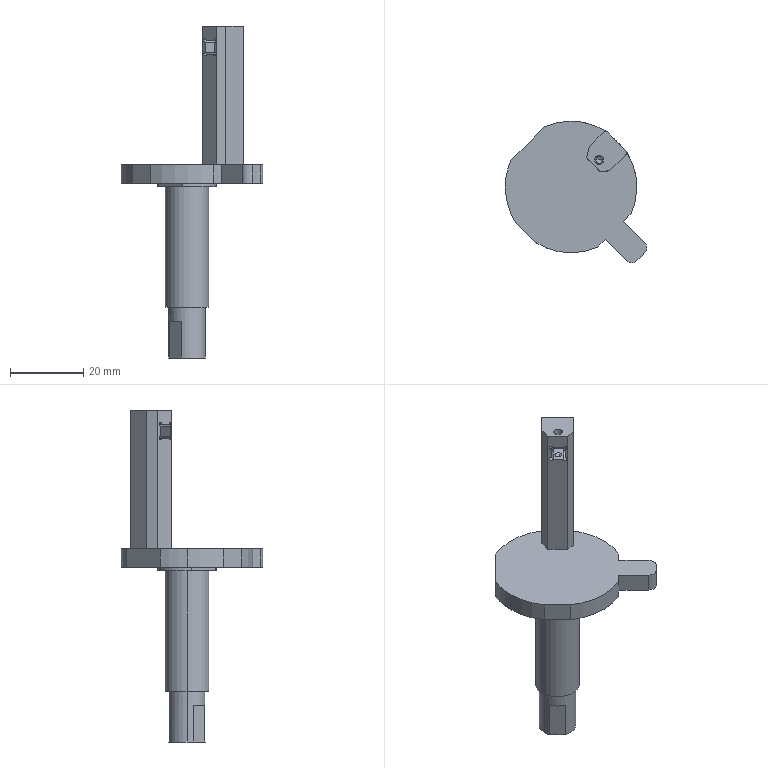Part | STEP file | 05-02 bending swing lever 1 | 1 solid | 66 faces | box 38.738 x 38.738 x 90.85 mm | volume 12920 mm3 | plane 34 | cylinder 30 | cone 2 | commonest cylinder face diameters 1 x6 12 x5 36 x5 2.5 x4 10 x4 4 x3